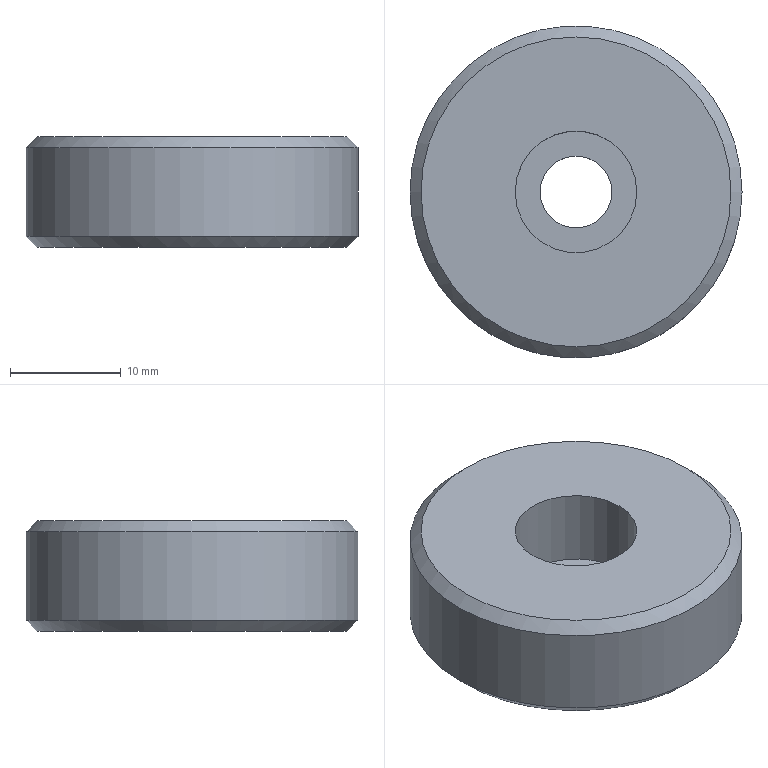Part | NX | features solid 2 | 1 solid | 8 faces | box 30 x 30 x 10 mm | volume 6212 mm3 | plane 3 | cylinder 3 | cone 2 | commonest cylinder face diameters 6.5 x1 11 x1 30 x1
STEP:
#1=CARTESIAN_POINT('',(14.,100.,-180.5));
#2=VERTEX_POINT('',#1);
#3=CARTESIAN_POINT('',(0.,100.,-180.5));
#4=DIRECTION('',(0.,0.,1.));
#5=DIRECTION('',(1.,0.,0.));
#6=AXIS2_PLACEMENT_3D('',#3,#4,#5);
#7=CIRCLE('',#6,14.);
#8=EDGE_CURVE('',#2,#2,#7,.T.);
#9=ORIENTED_EDGE('',*,*,#8,.T.);
#10=EDGE_LOOP('',(#9));
#11=FACE_BOUND('',#10,.T.);
#12=CARTESIAN_POINT('',(5.5,100.,-180.5));
#13=VERTEX_POINT('',#12);
#14=CARTESIAN_POINT('',(0.,100.,-180.5));
#15=DIRECTION('',(0.,0.,-1.));
#16=DIRECTION('',(1.,0.,0.));
#17=AXIS2_PLACEMENT_3D('',#14,#15,#16);
#18=CIRCLE('',#17,5.5);
#19=EDGE_CURVE('',#13,#13,#18,.T.);
#20=ORIENTED_EDGE('',*,*,#19,.T.);
#21=EDGE_LOOP('',(#20));
#22=FACE_BOUND('',#21,.T.);
#23=CARTESIAN_POINT('',(0.,100.,-180.5));
#24=DIRECTION('',(0.,0.,1.));
#25=DIRECTION('',(1.,0.,0.));
#26=AXIS2_PLACEMENT_3D('',#23,#24,#25);
#27=PLANE('',#26);
#28=ADVANCED_FACE('',(#11,#22),#27,.T.);
#29=CARTESIAN_POINT('',(-14.,100.,-190.5));
#30=VERTEX_POINT('',#29);
#31=CARTESIAN_POINT('',(0.,100.,-190.5));
#32=DIRECTION('',(0.,0.,-1.));
#33=DIRECTION('',(-1.,0.,0.));
#34=AXIS2_PLACEMENT_3D('',#31,#32,#33);
#35=CIRCLE('',#34,14.);
#36=EDGE_CURVE('',#30,#30,#35,.T.);
#37=ORIENTED_EDGE('',*,*,#36,.T.);
#38=EDGE_LOOP('',(#37));
#39=FACE_BOUND('',#38,.T.);
#40=CARTESIAN_POINT('',(3.25,100.,-190.5));
#41=VERTEX_POINT('',#40);
#42=CARTESIAN_POINT('',(0.,100.,-190.5));
#43=DIRECTION('',(0.,0.,1.));
#44=DIRECTION('',(1.,0.,0.));
#45=AXIS2_PLACEMENT_3D('',#42,#43,#44);
#46=CIRCLE('',#45,3.25);
#47=EDGE_CURVE('',#41,#41,#46,.T.);
#48=ORIENTED_EDGE('',*,*,#47,.T.);
#49=EDGE_LOOP('',(#48));
#50=FACE_BOUND('',#49,.T.);
#51=CARTESIAN_POINT('',(0.,100.,-190.5));
#52=DIRECTION('',(0.,0.,-1.));
#53=DIRECTION('',(-1.,0.,0.));
#54=AXIS2_PLACEMENT_3D('',#51,#52,#53);
#55=PLANE('',#54);
#56=ADVANCED_FACE('',(#39,#50),#55,.T.);
#57=CARTESIAN_POINT('',(-15.,100.,-189.5));
#58=VERTEX_POINT('',#57);
#59=CARTESIAN_POINT('',(0.,100.,-189.5));
#60=DIRECTION('',(0.,0.,-1.));
#61=DIRECTION('',(-1.,0.,0.));
#62=AXIS2_PLACEMENT_3D('',#59,#60,#61);
#63=CIRCLE('',#62,15.);
#64=EDGE_CURVE('',#58,#58,#63,.F.);
#65=ORIENTED_EDGE('',*,*,#64,.T.);
#66=EDGE_LOOP('',(#65));
#67=FACE_BOUND('',#66,.T.);
#68=CARTESIAN_POINT('',(15.,100.,-181.5));
#69=VERTEX_POINT('',#68);
#70=CARTESIAN_POINT('',(0.,100.,-181.5));
#71=DIRECTION('',(0.,0.,1.));
#72=DIRECTION('',(1.,0.,0.));
#73=AXIS2_PLACEMENT_3D('',#70,#71,#72);
#74=CIRCLE('',#73,15.);
#75=EDGE_CURVE('',#69,#69,#74,.F.);
#76=ORIENTED_EDGE('',*,*,#75,.T.);
#77=EDGE_LOOP('',(#76));
#78=FACE_BOUND('',#77,.T.);
#79=CARTESIAN_POINT('',(0.,100.,-190.5));
#80=DIRECTION('',(0.,0.,1.));
#81=DIRECTION('',(1.,0.,0.));
#82=AXIS2_PLACEMENT_3D('',#79,#80,#81);
#83=CYLINDRICAL_SURFACE('',#82,15.);
#84=ADVANCED_FACE('',(#67,#78),#83,.T.);
#85=CARTESIAN_POINT('',(-3.25,100.,-187.5));
#86=VERTEX_POINT('',#85);
#87=CARTESIAN_POINT('',(0.,100.,-187.5));
#88=DIRECTION('',(0.,0.,-1.));
#89=DIRECTION('',(-1.,0.,0.));
#90=AXIS2_PLACEMENT_3D('',#87,#88,#89);
#91=CIRCLE('',#90,3.25);
#92=EDGE_CURVE('',#86,#86,#91,.F.);
#93=ORIENTED_EDGE('',*,*,#92,.T.);
#94=EDGE_LOOP('',(#93));
#95=FACE_BOUND('',#94,.T.);
#96=ORIENTED_EDGE('',*,*,#47,.F.);
#97=EDGE_LOOP('',(#96));
#98=FACE_BOUND('',#97,.T.);
#99=CARTESIAN_POINT('',(0.,100.,-180.5));
#100=DIRECTION('',(0.,0.,-1.));
#101=DIRECTION('',(1.,0.,0.));
#102=AXIS2_PLACEMENT_3D('',#99,#100,#101);
#103=CYLINDRICAL_SURFACE('',#102,3.25);
#104=ADVANCED_FACE('',(#95,#98),#103,.F.);
#105=CARTESIAN_POINT('',(5.5,100.,-187.5));
#106=VERTEX_POINT('',#105);
#107=CARTESIAN_POINT('',(0.,100.,-187.5));
#108=DIRECTION('',(0.,0.,1.));
#109=DIRECTION('',(1.,0.,0.));
#110=AXIS2_PLACEMENT_3D('',#107,#108,#109);
#111=CIRCLE('',#110,5.5);
#112=EDGE_CURVE('',#106,#106,#111,.F.);
#113=ORIENTED_EDGE('',*,*,#112,.F.);
#114=EDGE_LOOP('',(#113));
#115=FACE_BOUND('',#114,.T.);
#116=ORIENTED_EDGE('',*,*,#92,.F.);
#117=EDGE_LOOP('',(#116));
#118=FACE_BOUND('',#117,.T.);
#119=CARTESIAN_POINT('',(0.,100.,-187.5));
#120=DIRECTION('',(0.,0.,-1.));
#121=DIRECTION('',(-1.,0.,0.));
#122=AXIS2_PLACEMENT_3D('',#119,#120,#121);
#123=PLANE('',#122);
#124=ADVANCED_FACE('',(#115,#118),#123,.F.);
#125=ORIENTED_EDGE('',*,*,#112,.T.);
#126=EDGE_LOOP('',(#125));
#127=FACE_BOUND('',#126,.T.);
#128=ORIENTED_EDGE('',*,*,#19,.F.);
#129=EDGE_LOOP('',(#128));
#130=FACE_BOUND('',#129,.T.);
#131=CARTESIAN_POINT('',(0.,100.,-180.5));
#132=DIRECTION('',(0.,0.,-1.));
#133=DIRECTION('',(1.,0.,0.));
#134=AXIS2_PLACEMENT_3D('',#131,#132,#133);
#135=CYLINDRICAL_SURFACE('',#134,5.5);
#136=ADVANCED_FACE('',(#127,#130),#135,.F.);
#137=ORIENTED_EDGE('',*,*,#36,.F.);
#138=EDGE_LOOP('',(#137));
#139=FACE_BOUND('',#138,.T.);
#140=ORIENTED_EDGE('',*,*,#64,.F.);
#141=EDGE_LOOP('',(#140));
#142=FACE_BOUND('',#141,.T.);
#143=CARTESIAN_POINT('',(0.,100.,-189.5));
#144=DIRECTION('',(0.,0.,1.));
#145=DIRECTION('',(1.,0.,0.));
#146=AXIS2_PLACEMENT_3D('',#143,#144,#145);
#147=CONICAL_SURFACE('',#146,15.,0.7854);
#148=ADVANCED_FACE('',(#139,#142),#147,.T.);
#149=ORIENTED_EDGE('',*,*,#8,.F.);
#150=EDGE_LOOP('',(#149));
#151=FACE_BOUND('',#150,.T.);
#152=ORIENTED_EDGE('',*,*,#75,.F.);
#153=EDGE_LOOP('',(#152));
#154=FACE_BOUND('',#153,.T.);
#155=CARTESIAN_POINT('',(0.,100.,-181.5));
#156=DIRECTION('',(0.,0.,-1.));
#157=DIRECTION('',(-1.,0.,0.));
#158=AXIS2_PLACEMENT_3D('',#155,#156,#157);
#159=CONICAL_SURFACE('',#158,15.,0.7854);
#160=ADVANCED_FACE('',(#151,#154),#159,.T.);
#161=CLOSED_SHELL('',(#28,#56,#84,#104,#124,#136,#148,#160));
#162=MANIFOLD_SOLID_BREP('',#161);
#163=(LENGTH_UNIT()NAMED_UNIT(*)SI_UNIT(.MILLI.,.METRE.));
#164=UNCERTAINTY_MEASURE_WITH_UNIT(LENGTH_MEASURE(0.00001),#163,'','');
#165=(NAMED_UNIT(*)PLANE_ANGLE_UNIT()SI_UNIT($,.RADIAN.));
#166=(NAMED_UNIT(*)SI_UNIT($,.STERADIAN.)SOLID_ANGLE_UNIT());
#167=(GEOMETRIC_REPRESENTATION_CONTEXT(3)GLOBAL_UNCERTAINTY_ASSIGNED_CONTEXT((#164))GLOBAL_UNIT_ASSIGNED_CONTEXT((#163,#165,#166))REPRESENTATION_CONTEXT('',''));
#168=ADVANCED_BREP_SHAPE_REPRESENTATION('',(#162),#167);